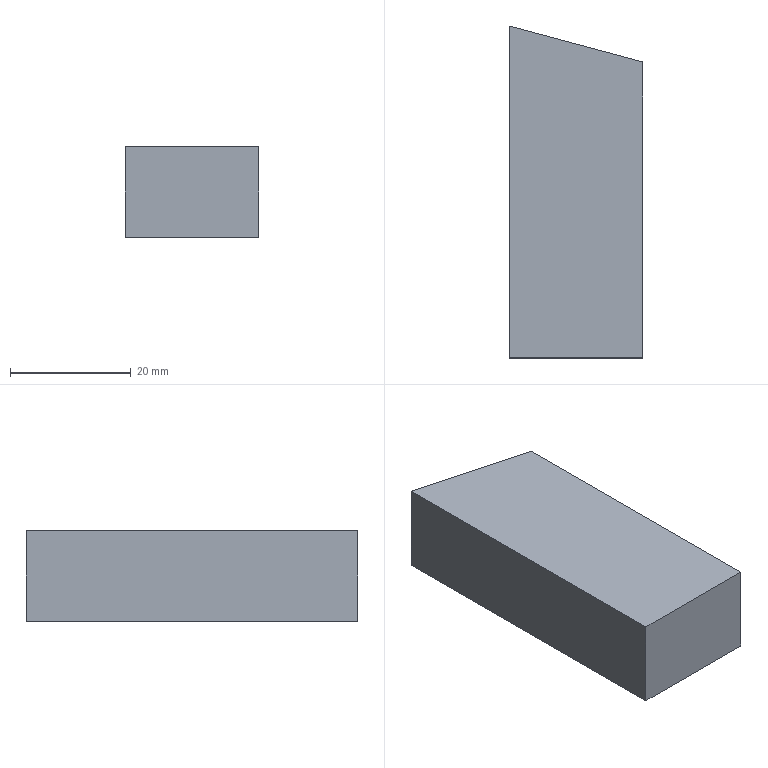Part | NX | features pipe injector 2 | 1 solid | 6 faces | box 22.2 x 55 x 15 mm | volume 17325 mm3 | plane 6
STEP:
#1=CARTESIAN_POINT('',(-22.2,-49.052,0.));
#2=VERTEX_POINT('',#1);
#3=CARTESIAN_POINT('',(-22.2,5.948,0.));
#4=VERTEX_POINT('',#3);
#5=CARTESIAN_POINT('',(-22.2,-49.052,0.));
#6=DIRECTION('',(0.,1.,0.));
#7=VECTOR('',#6,1000.);
#8=LINE('',#5,#7);
#9=EDGE_CURVE('',#2,#4,#8,.T.);
#10=ORIENTED_EDGE('',*,*,#9,.F.);
#11=CARTESIAN_POINT('',(0.,-49.052,0.));
#12=VERTEX_POINT('',#11);
#13=CARTESIAN_POINT('',(0.,-49.052,0.));
#14=DIRECTION('',(1.,0.,0.));
#15=VECTOR('',#14,1000.);
#16=LINE('',#13,#15);
#17=EDGE_CURVE('',#12,#2,#16,.F.);
#18=ORIENTED_EDGE('',*,*,#17,.F.);
#19=CARTESIAN_POINT('',(0.,0.,0.));
#20=VERTEX_POINT('',#19);
#21=CARTESIAN_POINT('',(0.,0.,0.));
#22=DIRECTION('',(0.,1.,0.));
#23=VECTOR('',#22,1000.);
#24=LINE('',#21,#23);
#25=EDGE_CURVE('',#20,#12,#24,.F.);
#26=ORIENTED_EDGE('',*,*,#25,.F.);
#27=CARTESIAN_POINT('',(-22.2,5.948,0.));
#28=DIRECTION('',(-0.9659,0.2588,0.));
#29=VECTOR('',#28,1000.);
#30=LINE('',#27,#29);
#31=EDGE_CURVE('',#4,#20,#30,.F.);
#32=ORIENTED_EDGE('',*,*,#31,.F.);
#33=EDGE_LOOP('',(#10,#18,#26,#32));
#34=FACE_BOUND('',#33,.T.);
#35=CARTESIAN_POINT('',(0.,0.,0.));
#36=DIRECTION('',(0.,0.,-1.));
#37=DIRECTION('',(-1.,0.,0.));
#38=AXIS2_PLACEMENT_3D('',#35,#36,#37);
#39=PLANE('',#38);
#40=ADVANCED_FACE('',(#34),#39,.F.);
#41=CARTESIAN_POINT('',(-22.2,5.948,-15.));
#42=VERTEX_POINT('',#41);
#43=CARTESIAN_POINT('',(0.,0.,-15.));
#44=VERTEX_POINT('',#43);
#45=CARTESIAN_POINT('',(-22.2,5.948,-15.));
#46=DIRECTION('',(0.9659,-0.2588,0.));
#47=VECTOR('',#46,1000.);
#48=LINE('',#45,#47);
#49=EDGE_CURVE('',#42,#44,#48,.T.);
#50=ORIENTED_EDGE('',*,*,#49,.F.);
#51=CARTESIAN_POINT('',(-22.2,5.948,-15.));
#52=DIRECTION('',(0.,0.,1.));
#53=VECTOR('',#52,1000.);
#54=LINE('',#51,#53);
#55=EDGE_CURVE('',#4,#42,#54,.F.);
#56=ORIENTED_EDGE('',*,*,#55,.F.);
#57=ORIENTED_EDGE('',*,*,#31,.T.);
#58=CARTESIAN_POINT('',(0.,0.,-15.));
#59=DIRECTION('',(0.,0.,1.));
#60=VECTOR('',#59,1000.);
#61=LINE('',#58,#60);
#62=EDGE_CURVE('',#44,#20,#61,.T.);
#63=ORIENTED_EDGE('',*,*,#62,.F.);
#64=EDGE_LOOP('',(#50,#56,#57,#63));
#65=FACE_BOUND('',#64,.T.);
#66=CARTESIAN_POINT('',(-22.2,5.948,-15.));
#67=DIRECTION('',(0.2588,0.9659,0.));
#68=DIRECTION('',(-0.9659,0.2588,0.));
#69=AXIS2_PLACEMENT_3D('',#66,#67,#68);
#70=PLANE('',#69);
#71=ADVANCED_FACE('',(#65),#70,.T.);
#72=CARTESIAN_POINT('',(0.,-49.052,-15.));
#73=VERTEX_POINT('',#72);
#74=CARTESIAN_POINT('',(0.,0.,-15.));
#75=DIRECTION('',(0.,1.,0.));
#76=VECTOR('',#75,1000.);
#77=LINE('',#74,#76);
#78=EDGE_CURVE('',#44,#73,#77,.F.);
#79=ORIENTED_EDGE('',*,*,#78,.F.);
#80=ORIENTED_EDGE('',*,*,#62,.T.);
#81=ORIENTED_EDGE('',*,*,#25,.T.);
#82=CARTESIAN_POINT('',(0.,-49.052,-15.));
#83=DIRECTION('',(0.,0.,-1.));
#84=VECTOR('',#83,1000.);
#85=LINE('',#82,#84);
#86=EDGE_CURVE('',#73,#12,#85,.F.);
#87=ORIENTED_EDGE('',*,*,#86,.F.);
#88=EDGE_LOOP('',(#79,#80,#81,#87));
#89=FACE_BOUND('',#88,.T.);
#90=CARTESIAN_POINT('',(0.,0.,-15.));
#91=DIRECTION('',(1.,0.,0.));
#92=DIRECTION('',(0.,1.,0.));
#93=AXIS2_PLACEMENT_3D('',#90,#91,#92);
#94=PLANE('',#93);
#95=ADVANCED_FACE('',(#89),#94,.T.);
#96=CARTESIAN_POINT('',(-22.2,-49.052,-15.));
#97=VERTEX_POINT('',#96);
#98=CARTESIAN_POINT('',(0.,-49.052,-15.));
#99=DIRECTION('',(-1.,0.,0.));
#100=VECTOR('',#99,1000.);
#101=LINE('',#98,#100);
#102=EDGE_CURVE('',#73,#97,#101,.T.);
#103=ORIENTED_EDGE('',*,*,#102,.F.);
#104=ORIENTED_EDGE('',*,*,#86,.T.);
#105=ORIENTED_EDGE('',*,*,#17,.T.);
#106=CARTESIAN_POINT('',(-22.2,-49.052,-15.));
#107=DIRECTION('',(0.,0.,1.));
#108=VECTOR('',#107,1000.);
#109=LINE('',#106,#108);
#110=EDGE_CURVE('',#97,#2,#109,.T.);
#111=ORIENTED_EDGE('',*,*,#110,.F.);
#112=EDGE_LOOP('',(#103,#104,#105,#111));
#113=FACE_BOUND('',#112,.T.);
#114=CARTESIAN_POINT('',(0.,-49.052,-15.));
#115=DIRECTION('',(0.,-1.,0.));
#116=DIRECTION('',(0.,0.,-1.));
#117=AXIS2_PLACEMENT_3D('',#114,#115,#116);
#118=PLANE('',#117);
#119=ADVANCED_FACE('',(#113),#118,.T.);
#120=CARTESIAN_POINT('',(-22.2,0.,-15.));
#121=DIRECTION('',(0.,1.,0.));
#122=VECTOR('',#121,1000.);
#123=LINE('',#120,#122);
#124=EDGE_CURVE('',#97,#42,#123,.T.);
#125=ORIENTED_EDGE('',*,*,#124,.F.);
#126=ORIENTED_EDGE('',*,*,#110,.T.);
#127=ORIENTED_EDGE('',*,*,#9,.T.);
#128=ORIENTED_EDGE('',*,*,#55,.T.);
#129=EDGE_LOOP('',(#125,#126,#127,#128));
#130=FACE_BOUND('',#129,.T.);
#131=CARTESIAN_POINT('',(-22.2,-49.052,-15.));
#132=DIRECTION('',(-1.,0.,0.));
#133=DIRECTION('',(0.,0.,1.));
#134=AXIS2_PLACEMENT_3D('',#131,#132,#133);
#135=PLANE('',#134);
#136=ADVANCED_FACE('',(#130),#135,.T.);
#137=ORIENTED_EDGE('',*,*,#102,.T.);
#138=ORIENTED_EDGE('',*,*,#124,.T.);
#139=ORIENTED_EDGE('',*,*,#49,.T.);
#140=ORIENTED_EDGE('',*,*,#78,.T.);
#141=EDGE_LOOP('',(#137,#138,#139,#140));
#142=FACE_BOUND('',#141,.T.);
#143=CARTESIAN_POINT('',(0.,0.,-15.));
#144=DIRECTION('',(0.,0.,-1.));
#145=DIRECTION('',(-1.,0.,0.));
#146=AXIS2_PLACEMENT_3D('',#143,#144,#145);
#147=PLANE('',#146);
#148=ADVANCED_FACE('',(#142),#147,.T.);
#149=CLOSED_SHELL('',(#40,#71,#95,#119,#136,#148));
#150=MANIFOLD_SOLID_BREP('',#149);
#151=(LENGTH_UNIT()NAMED_UNIT(*)SI_UNIT(.MILLI.,.METRE.));
#152=UNCERTAINTY_MEASURE_WITH_UNIT(LENGTH_MEASURE(0.00001),#151,'','');
#153=(NAMED_UNIT(*)PLANE_ANGLE_UNIT()SI_UNIT($,.RADIAN.));
#154=(NAMED_UNIT(*)SI_UNIT($,.STERADIAN.)SOLID_ANGLE_UNIT());
#155=(GEOMETRIC_REPRESENTATION_CONTEXT(3)GLOBAL_UNCERTAINTY_ASSIGNED_CONTEXT((#152))GLOBAL_UNIT_ASSIGNED_CONTEXT((#151,#153,#154))REPRESENTATION_CONTEXT('',''));
#156=ADVANCED_BREP_SHAPE_REPRESENTATION('',(#150),#155);